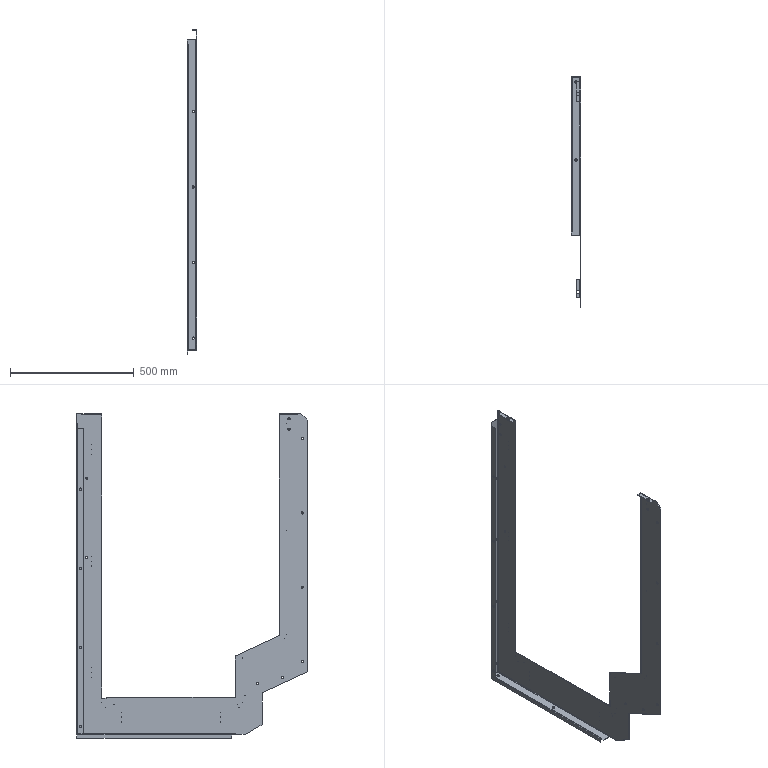Part | NX | features solid 2 | 1 solid | 184 faces | box 40 x 930 x 1310 mm | volume 969804 mm3 | cylinder 116 | plane 65 | spline 3 | commonest cylinder face diameters 1 x56 9.2 x32 8.1 x8 4 x6 8 x6 10 x4